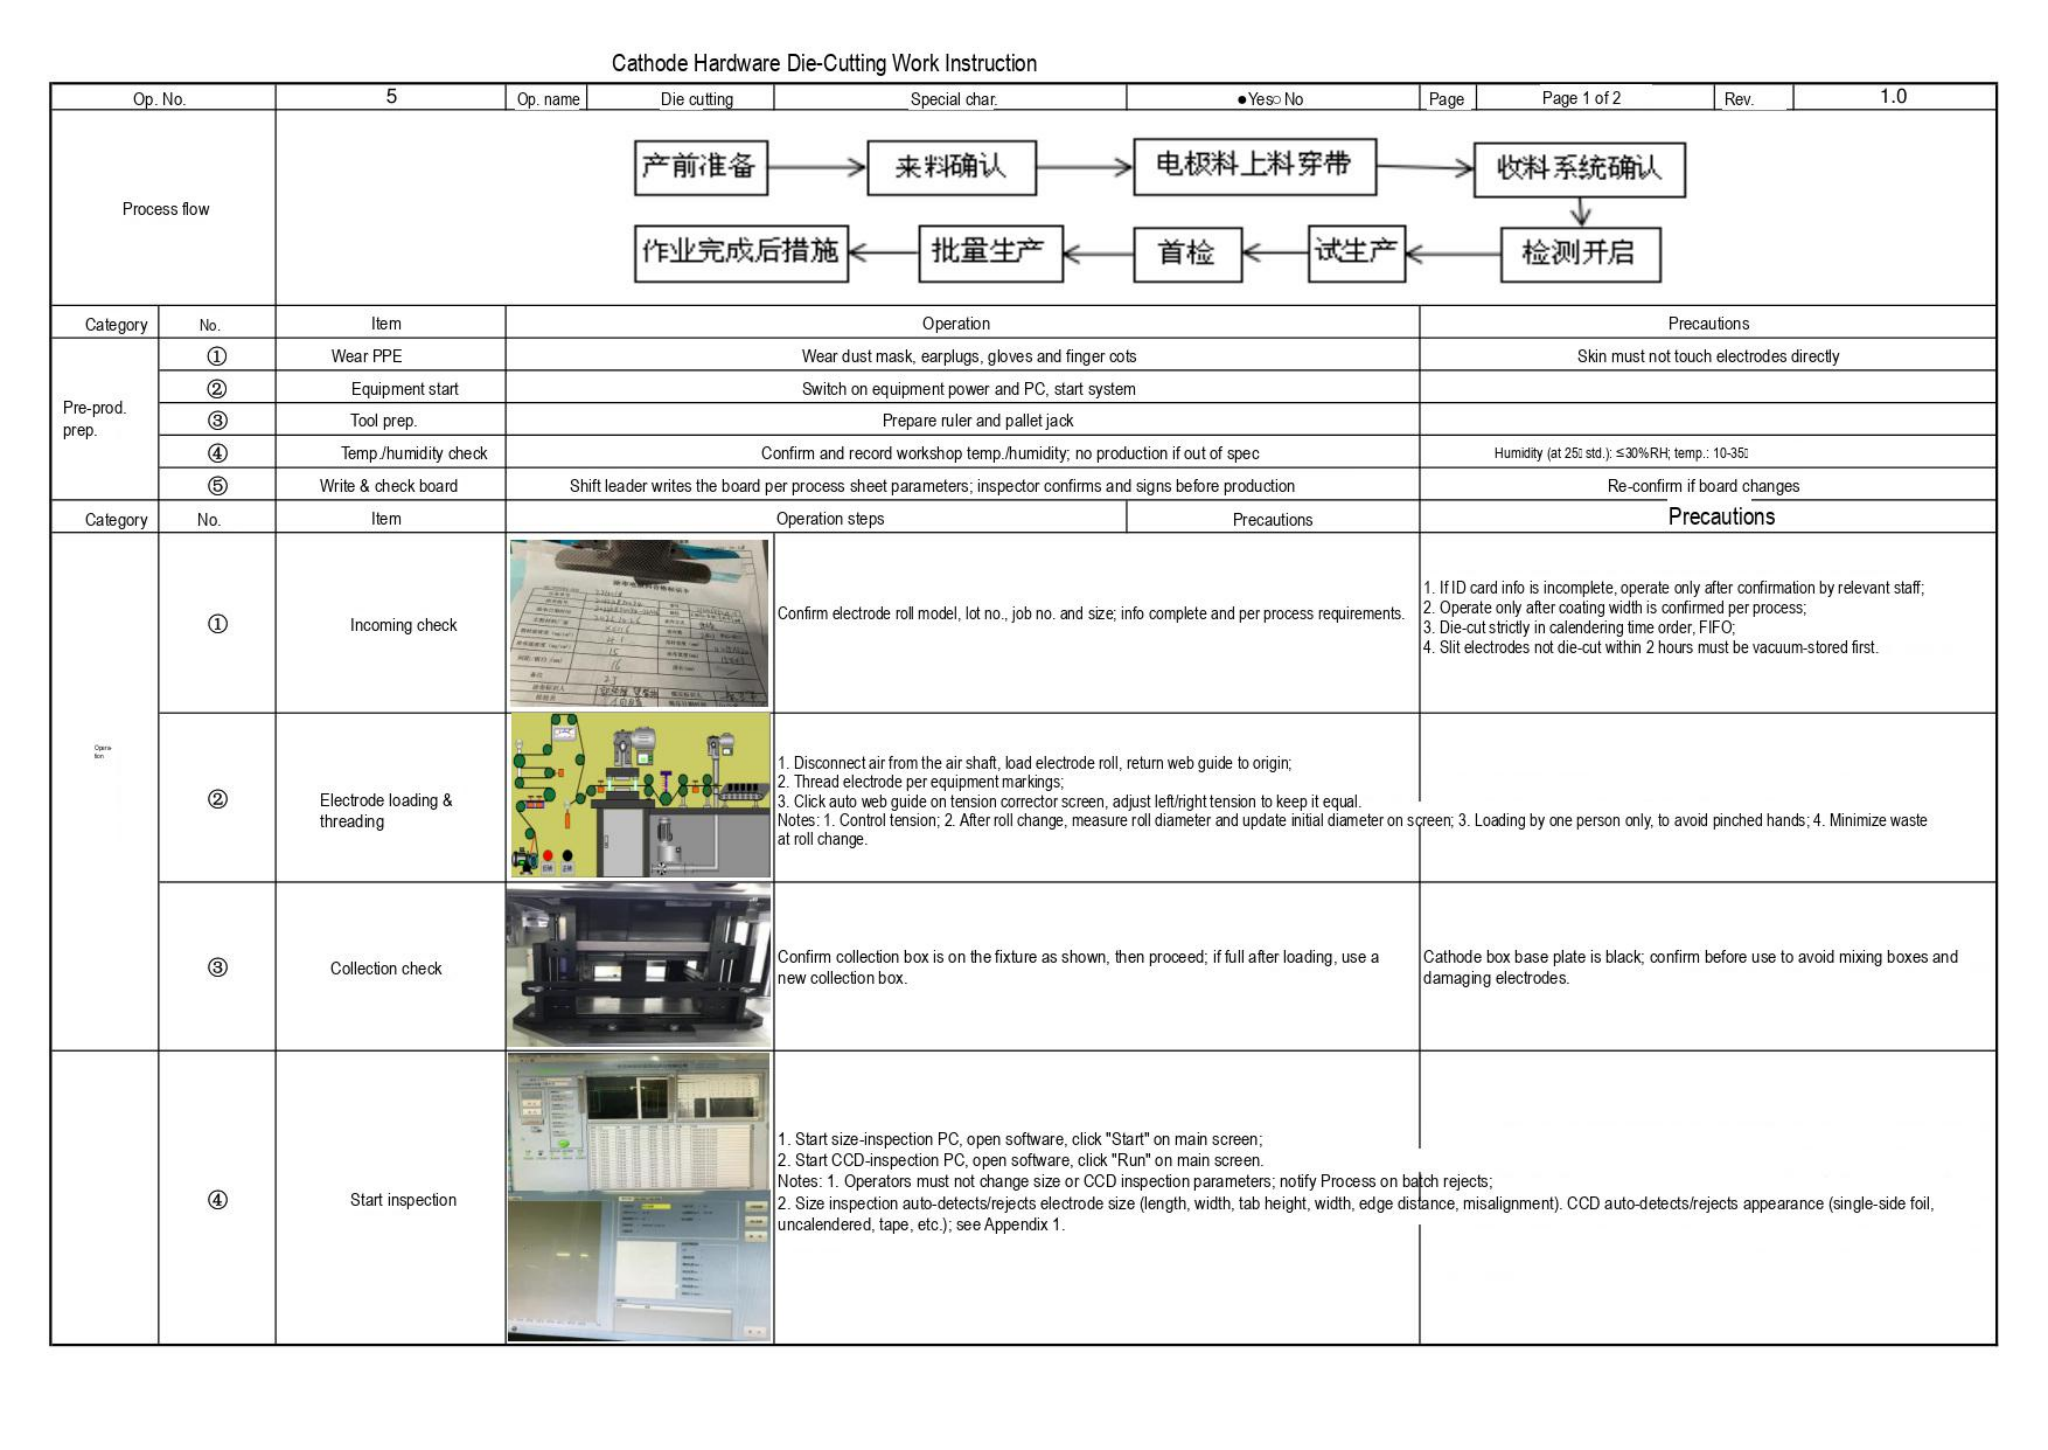Cathode Hardware Die-Cutting Work Instruction

| Op. No. | 5 | Op. name | Die cutting | Special char. | ●Yes○ No | Page | Page 1 of 2 | Rev. | 1.0 |
|---|---|---|---|---|---|---|---|---|---|

**Process flow**

产前准备 → 来料确认 → 电极料上料穿带 → 收料系统确认
↓
作业完成后措施 ← 批量生产 ← 首检 ← 试生产 ← 检测开启

| Category | No. | Item | Operation | Precautions |
|---|---|---|---|---|
| Pre-prod. prep. | ① | Wear PPE | Wear dust mask, earplugs, gloves and finger cots | Skin must not touch electrodes directly |
| | ② | Equipment start | Switch on equipment power and PC, start system | |
| | ③ | Tool prep. | Prepare ruler and pallet jack | |
| | ④ | Temp./humidity check | Confirm and record workshop temp./humidity; no production if out of spec | Humidity (at 25 std.): ≤30%RH; temp.: 10-35 |
| | ⑤ | Write & check board | Shift leader writes the board per process sheet parameters; inspector confirms and signs before production | Re-confirm if board changes |

| Category | No. | Item | Operation steps | Precautions | Precautions |
|---|---|---|---|---|---|
| Opera tion | ① | Incoming check | Confirm electrode roll model, lot no., job no. and size; info complete and per process requirements. | | 1. If ID card info is incomplete, operate only after confirmation by relevant staff;<br>2. Operate only after coating width is confirmed per process;<br>3. Die-cut strictly in calendering time order, FIFO;<br>4. Slit electrodes not die-cut within 2 hours must be vacuum-stored first. |
| | ② | Electrode loading & threading | 1. Disconnect air from the air shaft, load electrode roll, return web guide to origin;<br>2. Thread electrode per equipment markings;<br>3. Click auto web guide on tension corrector screen, adjust left/right tension to keep it equal.<br>Notes: 1. Control tension; 2. After roll change, measure roll diameter and update initial diameter on screen; 3. Loading by one person only, to avoid pinched hands; 4. Minimize waste at roll change. | | |
| | ③ | Collection check | Confirm collection box is on the fixture as shown, then proceed; if full after loading, use a new collection box. | | Cathode box base plate is black; confirm before use to avoid mixing boxes and damaging electrodes. |
| | ④ | Start inspection | 1. Start size-inspection PC, open software, click "Start" on main screen;<br>2. Start CCD-inspection PC, open software, click "Run" on main screen.<br>Notes: 1. Operators must not change size or CCD inspection parameters; notify Process on batch rejects;<br>2. Size inspection auto-detects/rejects electrode size (length, width, tab height, width, edge distance, misalignment). CCD auto-detects/rejects appearance (single-side foil, uncalendered, tape, etc.); see Appendix 1. | | |
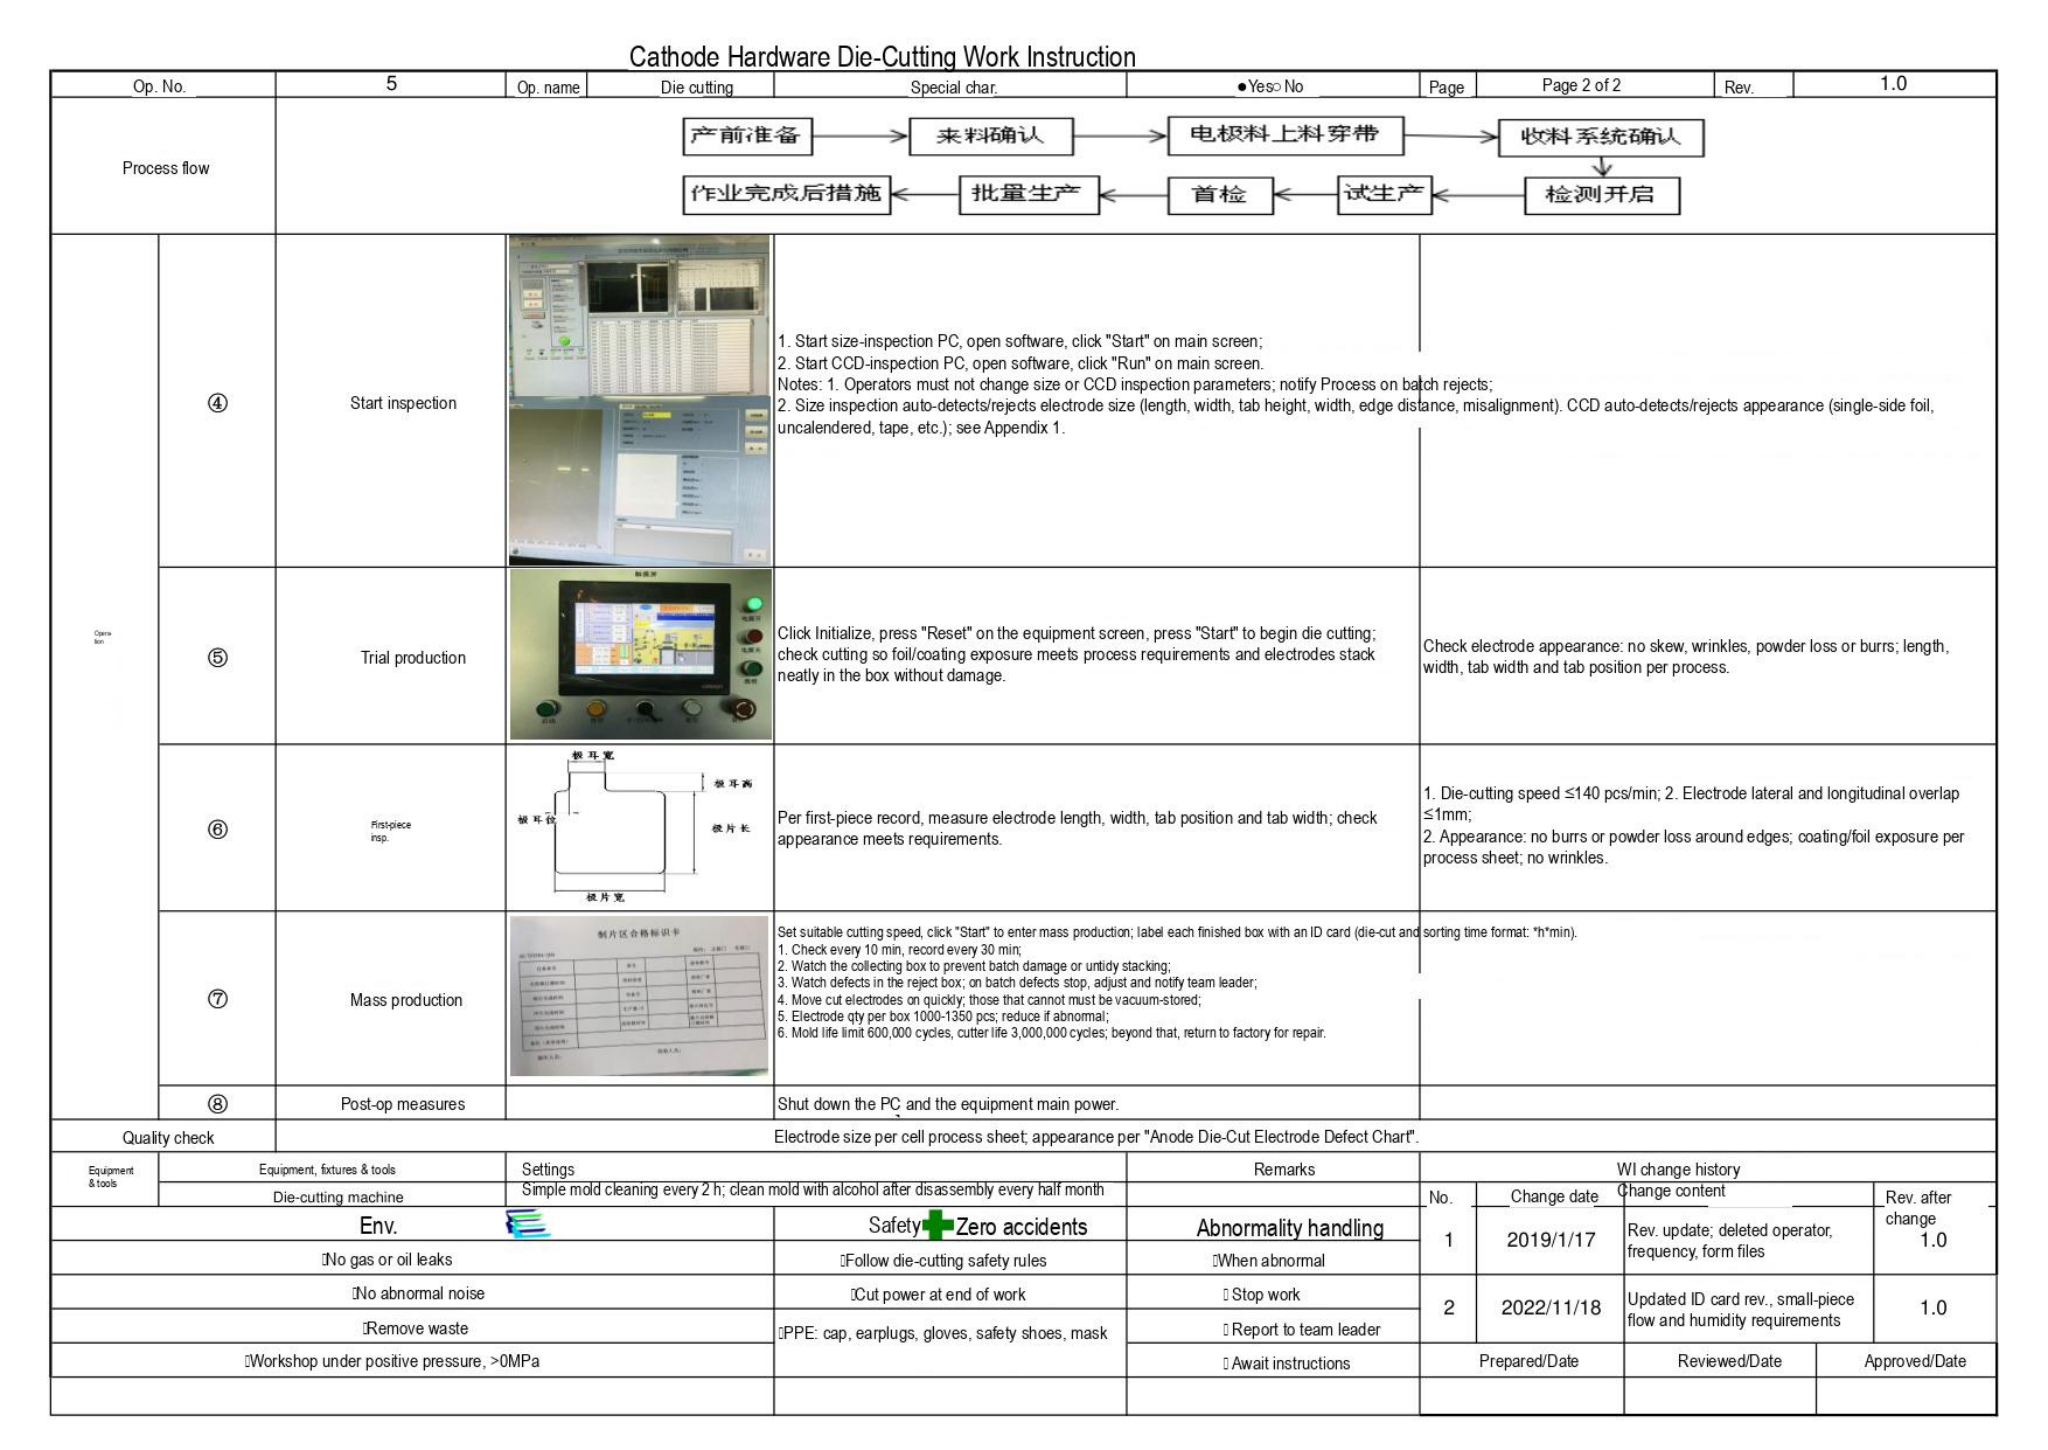# Cathode Hardware Die-Cutting Work Instruction

| Op. No. | 5 | Op. name | Die cutting | Special char. | ●Yes○No | Page | Page 2 of 2 | Rev. | 1.0 |
|---|---|---|---|---|---|---|---|---|---|

| Process flow | 产前准备 → 来料确认 → 电极料上料穿带 → 收料系统确认 → 检测开启 → 试生产 → 首检 → 批量生产 → 作业完成后措施 |
|---|---|

| Opera-tion | | | | | |
|---|---|---|---|---|---|
| | ④ | Start inspection | | 1. Start size-inspection PC, open software, click "Start" on main screen;<br>2. Start CCD-inspection PC, open software, click "Run" on main screen.<br>Notes: 1. Operators must not change size or CCD inspection parameters; notify Process on batch rejects;<br>2. Size inspection auto-detects/rejects electrode size (length, width, tab height, width, edge distance, misalignment). CCD auto-detects/rejects appearance (single-side foil, uncalendered, tape, etc.); see Appendix 1. | |
| | ⑤ | Trial production | | Click Initialize, press "Reset" on the equipment screen, press "Start" to begin die cutting; check cutting so foil/coating exposure meets process requirements and electrodes stack neatly in the box without damage. | Check electrode appearance: no skew, wrinkles, powder loss or burrs; length, width, tab width and tab position per process. |
| | ⑥ | First-piece insp. | 极耳宽<br>极耳高<br>极耳位<br>极片长<br>极片宽 | Per first-piece record, measure electrode length, width, tab position and tab width; check appearance meets requirements. | 1. Die-cutting speed ≤140 pcs/min; 2. Electrode lateral and longitudinal overlap ≤1mm;<br>2. Appearance: no burrs or powder loss around edges; coating/foil exposure per process sheet; no wrinkles. |
| | ⑦ | Mass production | 制片区合格标识卡 | Set suitable cutting speed, click "Start" to enter mass production; label each finished box with an ID card (die-cut and sorting time format: *h*min).<br>1. Check every 10 min, record every 30 min;<br>2. Watch the collecting box to prevent batch damage or untidy stacking;<br>3. Watch defects in the reject box; on batch defects stop, adjust and notify team leader;<br>4. Move cut electrodes on quickly; those that cannot must be vacuum-stored;<br>5. Electrode qty per box 1000-1350 pcs; reduce if abnormal;<br>6. Mold life limit 600,000 cycles, cutter life 3,000,000 cycles; beyond that, return to factory for repair. | |
| | ⑧ | Post-op measures | | Shut down the PC and the equipment main power. | |

| Quality check | Electrode size per cell process sheet; appearance per "Anode Die-Cut Electrode Defect Chart". |
|---|---|

| Equipment & tools | Equipment, fixtures & tools | Settings | Remarks |
|---|---|---|---|
| | Die-cutting machine | Simple mold cleaning every 2 h; clean mold with alcohol after disassembly every half month | |

| Env. | Safety Zero accidents | Abnormality handling |
|---|---|---|
| No gas or oil leaks | Follow die-cutting safety rules | When abnormal |
| No abnormal noise | Cut power at end of work | Stop work |
| Remove waste | PPE: cap, earplugs, gloves, safety shoes, mask | Report to team leader |
| Workshop under positive pressure, >0MPa | | Await instructions |

WI change history

| No. | Change date | Change content | Rev. after change |
|---|---|---|---|
| 1 | 2019/1/17 | Rev. update; deleted operator, frequency, form files | 1.0 |
| 2 | 2022/11/18 | Updated ID card rev., small-piece flow and humidity requirements | 1.0 |

| Prepared/Date | Reviewed/Date | Approved/Date |
|---|---|---|
| | | |